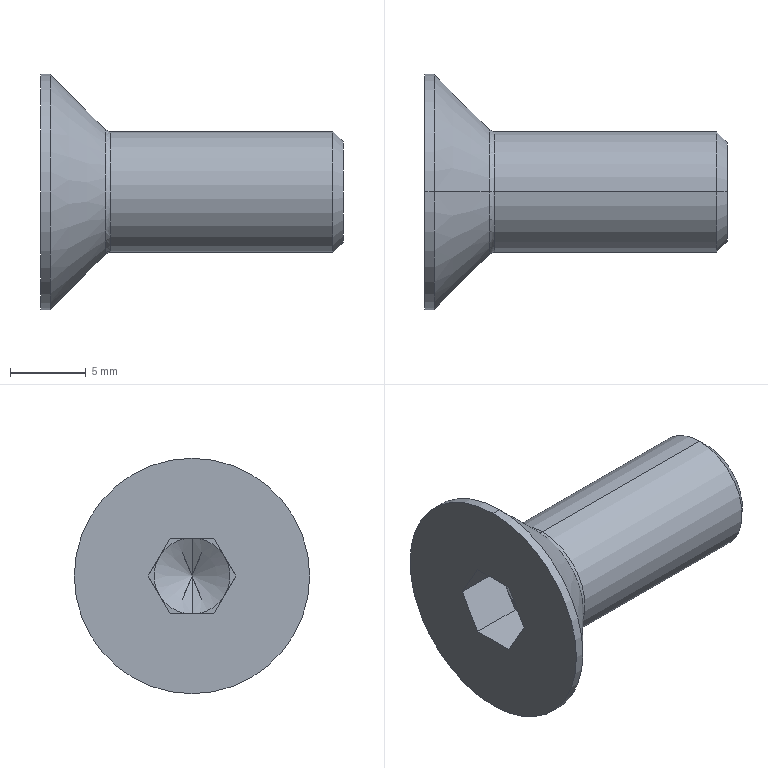Part | STEP file | socket countersunk head screw_din_DIN 7991 - M8 x 20 --- 11.8N | 1 solid | 26 faces | box 20 x 15.57 x 15.57 mm | volume 1237 mm3 | plane 14 | cone 6 | cylinder 4 | torus 2 | commonest cylinder face diameters 8 x2 15.57 x2